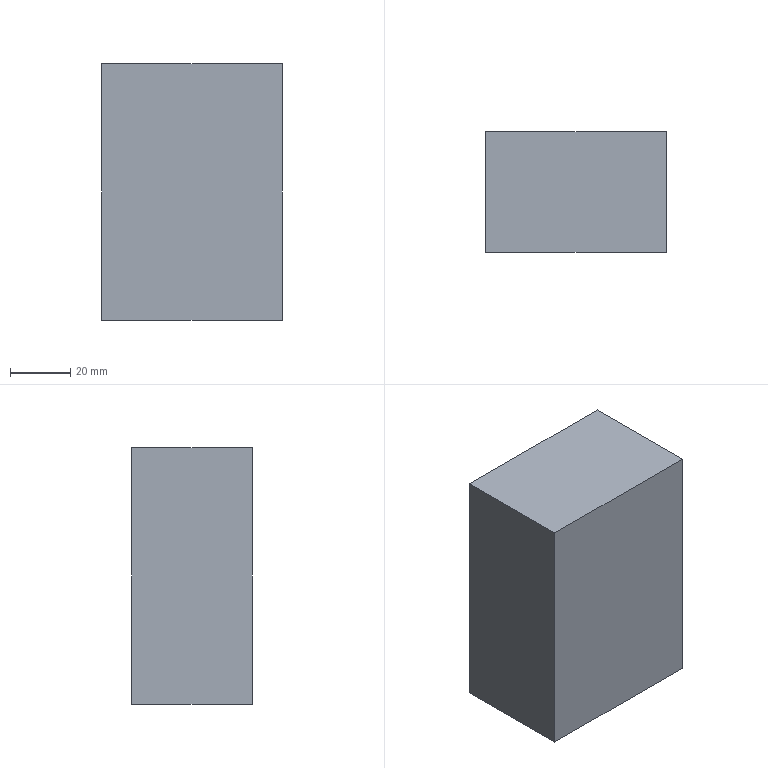Part | NX | features solid 2 | 1 solid | 10 faces | box 60 x 40 x 85 mm | volume 198298 mm3 | plane 8 | cylinder 2 | commonest cylinder face diameters 11 x2
STEP:
#1=CARTESIAN_POINT('',(647.5,-200.,35.));
#2=VERTEX_POINT('',#1);
#3=CARTESIAN_POINT('',(587.5,-200.,35.));
#4=VERTEX_POINT('',#3);
#5=CARTESIAN_POINT('',(647.5,-200.,35.));
#6=DIRECTION('',(-1.,0.,0.));
#7=VECTOR('',#6,1000.);
#8=LINE('',#5,#7);
#9=EDGE_CURVE('',#2,#4,#8,.T.);
#10=ORIENTED_EDGE('',*,*,#9,.F.);
#11=CARTESIAN_POINT('',(647.5,-160.,35.));
#12=VERTEX_POINT('',#11);
#13=CARTESIAN_POINT('',(647.5,-165.,35.));
#14=DIRECTION('',(0.,-1.,0.));
#15=VECTOR('',#14,1000.);
#16=LINE('',#13,#15);
#17=EDGE_CURVE('',#12,#2,#16,.T.);
#18=ORIENTED_EDGE('',*,*,#17,.F.);
#19=CARTESIAN_POINT('',(587.5,-160.,35.));
#20=VERTEX_POINT('',#19);
#21=CARTESIAN_POINT('',(647.5,-160.,35.));
#22=DIRECTION('',(-1.,0.,0.));
#23=VECTOR('',#22,1000.);
#24=LINE('',#21,#23);
#25=EDGE_CURVE('',#20,#12,#24,.F.);
#26=ORIENTED_EDGE('',*,*,#25,.F.);
#27=CARTESIAN_POINT('',(587.5,-180.,35.));
#28=DIRECTION('',(0.,1.,0.));
#29=VECTOR('',#28,1000.);
#30=LINE('',#27,#29);
#31=EDGE_CURVE('',#4,#20,#30,.T.);
#32=ORIENTED_EDGE('',*,*,#31,.F.);
#33=EDGE_LOOP('',(#10,#18,#26,#32));
#34=FACE_BOUND('',#33,.T.);
#35=CARTESIAN_POINT('',(587.5,-200.,35.));
#36=DIRECTION('',(0.,0.,-1.));
#37=DIRECTION('',(1.,0.,0.));
#38=AXIS2_PLACEMENT_3D('',#35,#36,#37);
#39=PLANE('',#38);
#40=ADVANCED_FACE('',(#34),#39,.F.);
#41=CARTESIAN_POINT('',(638.,-180.,-20.));
#42=VERTEX_POINT('',#41);
#43=CARTESIAN_POINT('',(632.5,-180.,-20.));
#44=DIRECTION('',(0.,0.,1.));
#45=DIRECTION('',(1.,0.,0.));
#46=AXIS2_PLACEMENT_3D('',#43,#44,#45);
#47=CIRCLE('',#46,5.5);
#48=EDGE_CURVE('',#42,#42,#47,.T.);
#49=ORIENTED_EDGE('',*,*,#48,.T.);
#50=EDGE_LOOP('',(#49));
#51=FACE_BOUND('',#50,.T.);
#52=CARTESIAN_POINT('',(627.,-180.,-50.));
#53=VERTEX_POINT('',#52);
#54=CARTESIAN_POINT('',(632.5,-180.,-50.));
#55=DIRECTION('',(0.,0.,-1.));
#56=DIRECTION('',(-1.,0.,0.));
#57=AXIS2_PLACEMENT_3D('',#54,#55,#56);
#58=CIRCLE('',#57,5.5);
#59=EDGE_CURVE('',#53,#53,#58,.F.);
#60=ORIENTED_EDGE('',*,*,#59,.F.);
#61=EDGE_LOOP('',(#60));
#62=FACE_BOUND('',#61,.T.);
#63=CARTESIAN_POINT('',(632.5,-180.,35.));
#64=DIRECTION('',(0.,0.,-1.));
#65=DIRECTION('',(1.,0.,0.));
#66=AXIS2_PLACEMENT_3D('',#63,#64,#65);
#67=CYLINDRICAL_SURFACE('',#66,5.5);
#68=ADVANCED_FACE('',(#51,#62),#67,.F.);
#69=ORIENTED_EDGE('',*,*,#17,.T.);
#70=CARTESIAN_POINT('',(647.5,-200.,-50.));
#71=VERTEX_POINT('',#70);
#72=CARTESIAN_POINT('',(647.5,-200.,-40.));
#73=DIRECTION('',(0.,0.,1.));
#74=VECTOR('',#73,1000.);
#75=LINE('',#72,#74);
#76=EDGE_CURVE('',#71,#2,#75,.T.);
#77=ORIENTED_EDGE('',*,*,#76,.F.);
#78=CARTESIAN_POINT('',(647.5,-160.,-50.));
#79=VERTEX_POINT('',#78);
#80=CARTESIAN_POINT('',(647.5,-165.,-50.));
#81=DIRECTION('',(0.,1.,0.));
#82=VECTOR('',#81,1000.);
#83=LINE('',#80,#82);
#84=EDGE_CURVE('',#79,#71,#83,.F.);
#85=ORIENTED_EDGE('',*,*,#84,.F.);
#86=CARTESIAN_POINT('',(647.5,-160.,-40.));
#87=DIRECTION('',(0.,0.,-1.));
#88=VECTOR('',#87,1000.);
#89=LINE('',#86,#88);
#90=EDGE_CURVE('',#12,#79,#89,.T.);
#91=ORIENTED_EDGE('',*,*,#90,.F.);
#92=EDGE_LOOP('',(#69,#77,#85,#91));
#93=FACE_BOUND('',#92,.T.);
#94=CARTESIAN_POINT('',(647.5,-165.,-40.));
#95=DIRECTION('',(1.,0.,0.));
#96=DIRECTION('',(0.,0.,1.));
#97=AXIS2_PLACEMENT_3D('',#94,#95,#96);
#98=PLANE('',#97);
#99=ADVANCED_FACE('',(#93),#98,.T.);
#100=ORIENTED_EDGE('',*,*,#84,.T.);
#101=CARTESIAN_POINT('',(587.5,-200.,-50.));
#102=VERTEX_POINT('',#101);
#103=CARTESIAN_POINT('',(137.5,-200.,-50.));
#104=DIRECTION('',(-1.,0.,0.));
#105=VECTOR('',#104,1000.);
#106=LINE('',#103,#105);
#107=EDGE_CURVE('',#102,#71,#106,.F.);
#108=ORIENTED_EDGE('',*,*,#107,.F.);
#109=CARTESIAN_POINT('',(587.5,-160.,-50.));
#110=VERTEX_POINT('',#109);
#111=CARTESIAN_POINT('',(587.5,-165.,-50.));
#112=DIRECTION('',(0.,1.,0.));
#113=VECTOR('',#112,1000.);
#114=LINE('',#111,#113);
#115=EDGE_CURVE('',#110,#102,#114,.F.);
#116=ORIENTED_EDGE('',*,*,#115,.F.);
#117=CARTESIAN_POINT('',(647.5,-160.,-50.));
#118=DIRECTION('',(1.,0.,0.));
#119=VECTOR('',#118,1000.);
#120=LINE('',#117,#119);
#121=EDGE_CURVE('',#110,#79,#120,.T.);
#122=ORIENTED_EDGE('',*,*,#121,.T.);
#123=EDGE_LOOP('',(#100,#108,#116,#122));
#124=FACE_BOUND('',#123,.T.);
#125=ORIENTED_EDGE('',*,*,#59,.T.);
#126=EDGE_LOOP('',(#125));
#127=FACE_BOUND('',#126,.T.);
#128=CARTESIAN_POINT('',(602.,-180.,-50.));
#129=VERTEX_POINT('',#128);
#130=CARTESIAN_POINT('',(607.5,-180.,-50.));
#131=DIRECTION('',(0.,0.,-1.));
#132=DIRECTION('',(-1.,0.,0.));
#133=AXIS2_PLACEMENT_3D('',#130,#131,#132);
#134=CIRCLE('',#133,5.5);
#135=EDGE_CURVE('',#129,#129,#134,.F.);
#136=ORIENTED_EDGE('',*,*,#135,.T.);
#137=EDGE_LOOP('',(#136));
#138=FACE_BOUND('',#137,.T.);
#139=CARTESIAN_POINT('',(137.5,-165.,-50.));
#140=DIRECTION('',(0.,0.,1.));
#141=DIRECTION('',(0.,-1.,0.));
#142=AXIS2_PLACEMENT_3D('',#139,#140,#141);
#143=PLANE('',#142);
#144=ADVANCED_FACE('',(#124,#127,#138),#143,.F.);
#145=ORIENTED_EDGE('',*,*,#76,.T.);
#146=ORIENTED_EDGE('',*,*,#9,.T.);
#147=CARTESIAN_POINT('',(587.5,-200.,-40.));
#148=DIRECTION('',(0.,0.,1.));
#149=VECTOR('',#148,1000.);
#150=LINE('',#147,#149);
#151=EDGE_CURVE('',#102,#4,#150,.T.);
#152=ORIENTED_EDGE('',*,*,#151,.F.);
#153=ORIENTED_EDGE('',*,*,#107,.T.);
#154=EDGE_LOOP('',(#145,#146,#152,#153));
#155=FACE_BOUND('',#154,.T.);
#156=CARTESIAN_POINT('',(647.5,-200.,-40.));
#157=DIRECTION('',(0.,-1.,0.));
#158=DIRECTION('',(0.,0.,1.));
#159=AXIS2_PLACEMENT_3D('',#156,#157,#158);
#160=PLANE('',#159);
#161=ADVANCED_FACE('',(#155),#160,.T.);
#162=ORIENTED_EDGE('',*,*,#90,.T.);
#163=ORIENTED_EDGE('',*,*,#121,.F.);
#164=CARTESIAN_POINT('',(587.5,-160.,-40.));
#165=DIRECTION('',(0.,0.,1.));
#166=VECTOR('',#165,1000.);
#167=LINE('',#164,#166);
#168=EDGE_CURVE('',#20,#110,#167,.F.);
#169=ORIENTED_EDGE('',*,*,#168,.F.);
#170=ORIENTED_EDGE('',*,*,#25,.T.);
#171=EDGE_LOOP('',(#162,#163,#169,#170));
#172=FACE_BOUND('',#171,.T.);
#173=CARTESIAN_POINT('',(647.5,-160.,-40.));
#174=DIRECTION('',(0.,-1.,0.));
#175=DIRECTION('',(0.,0.,1.));
#176=AXIS2_PLACEMENT_3D('',#173,#174,#175);
#177=PLANE('',#176);
#178=ADVANCED_FACE('',(#172),#177,.F.);
#179=ORIENTED_EDGE('',*,*,#31,.T.);
#180=ORIENTED_EDGE('',*,*,#168,.T.);
#181=ORIENTED_EDGE('',*,*,#115,.T.);
#182=ORIENTED_EDGE('',*,*,#151,.T.);
#183=EDGE_LOOP('',(#179,#180,#181,#182));
#184=FACE_BOUND('',#183,.T.);
#185=CARTESIAN_POINT('',(587.5,-180.,-33.221));
#186=DIRECTION('',(-1.,0.,0.));
#187=DIRECTION('',(0.,0.,-1.));
#188=AXIS2_PLACEMENT_3D('',#185,#186,#187);
#189=PLANE('',#188);
#190=ADVANCED_FACE('',(#184),#189,.T.);
#191=CARTESIAN_POINT('',(613.,-180.,-20.));
#192=VERTEX_POINT('',#191);
#193=CARTESIAN_POINT('',(607.5,-180.,-20.));
#194=DIRECTION('',(0.,0.,1.));
#195=DIRECTION('',(1.,0.,0.));
#196=AXIS2_PLACEMENT_3D('',#193,#194,#195);
#197=CIRCLE('',#196,5.5);
#198=EDGE_CURVE('',#192,#192,#197,.T.);
#199=ORIENTED_EDGE('',*,*,#198,.T.);
#200=EDGE_LOOP('',(#199));
#201=FACE_BOUND('',#200,.T.);
#202=ORIENTED_EDGE('',*,*,#135,.F.);
#203=EDGE_LOOP('',(#202));
#204=FACE_BOUND('',#203,.T.);
#205=CARTESIAN_POINT('',(607.5,-180.,35.));
#206=DIRECTION('',(0.,0.,-1.));
#207=DIRECTION('',(1.,0.,0.));
#208=AXIS2_PLACEMENT_3D('',#205,#206,#207);
#209=CYLINDRICAL_SURFACE('',#208,5.5);
#210=ADVANCED_FACE('',(#201,#204),#209,.F.);
#211=ORIENTED_EDGE('',*,*,#48,.F.);
#212=EDGE_LOOP('',(#211));
#213=FACE_BOUND('',#212,.T.);
#214=CARTESIAN_POINT('',(632.5,-180.,-20.));
#215=DIRECTION('',(0.,0.,-1.));
#216=DIRECTION('',(1.,0.,0.));
#217=AXIS2_PLACEMENT_3D('',#214,#215,#216);
#218=PLANE('',#217);
#219=ADVANCED_FACE('',(#213),#218,.T.);
#220=ORIENTED_EDGE('',*,*,#198,.F.);
#221=EDGE_LOOP('',(#220));
#222=FACE_BOUND('',#221,.T.);
#223=CARTESIAN_POINT('',(607.5,-180.,-20.));
#224=DIRECTION('',(0.,0.,-1.));
#225=DIRECTION('',(1.,0.,0.));
#226=AXIS2_PLACEMENT_3D('',#223,#224,#225);
#227=PLANE('',#226);
#228=ADVANCED_FACE('',(#222),#227,.T.);
#229=CLOSED_SHELL('',(#40,#68,#99,#144,#161,#178,#190,#210,#219,#228));
#230=MANIFOLD_SOLID_BREP('',#229);
#231=(LENGTH_UNIT()NAMED_UNIT(*)SI_UNIT(.MILLI.,.METRE.));
#232=UNCERTAINTY_MEASURE_WITH_UNIT(LENGTH_MEASURE(0.00001),#231,'','');
#233=(NAMED_UNIT(*)PLANE_ANGLE_UNIT()SI_UNIT($,.RADIAN.));
#234=(NAMED_UNIT(*)SI_UNIT($,.STERADIAN.)SOLID_ANGLE_UNIT());
#235=(GEOMETRIC_REPRESENTATION_CONTEXT(3)GLOBAL_UNCERTAINTY_ASSIGNED_CONTEXT((#232))GLOBAL_UNIT_ASSIGNED_CONTEXT((#231,#233,#234))REPRESENTATION_CONTEXT('',''));
#236=ADVANCED_BREP_SHAPE_REPRESENTATION('',(#230),#235);